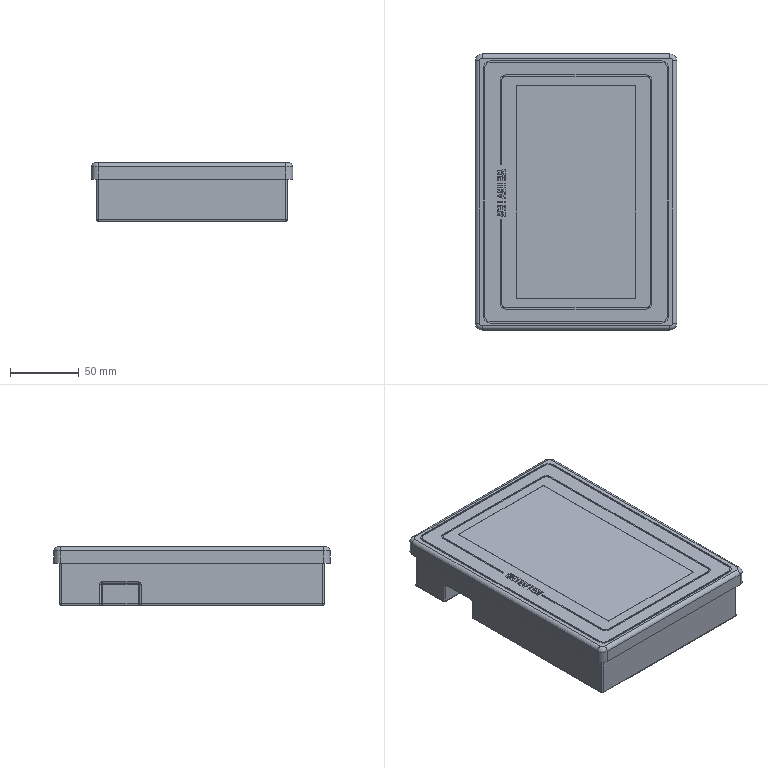Part | SolidWorks | features ICE 7, Fillet 3, Extrusion 1 | 1 solid | 191 faces | box 146.35 x 200.35 x 42.55 mm | volume 1144321 mm3 | plane 131 | cylinder 44 | sphere 8 | torus 8 | commonest cylinder face diameters 2 x20 6 x8 8 x8 10 x8